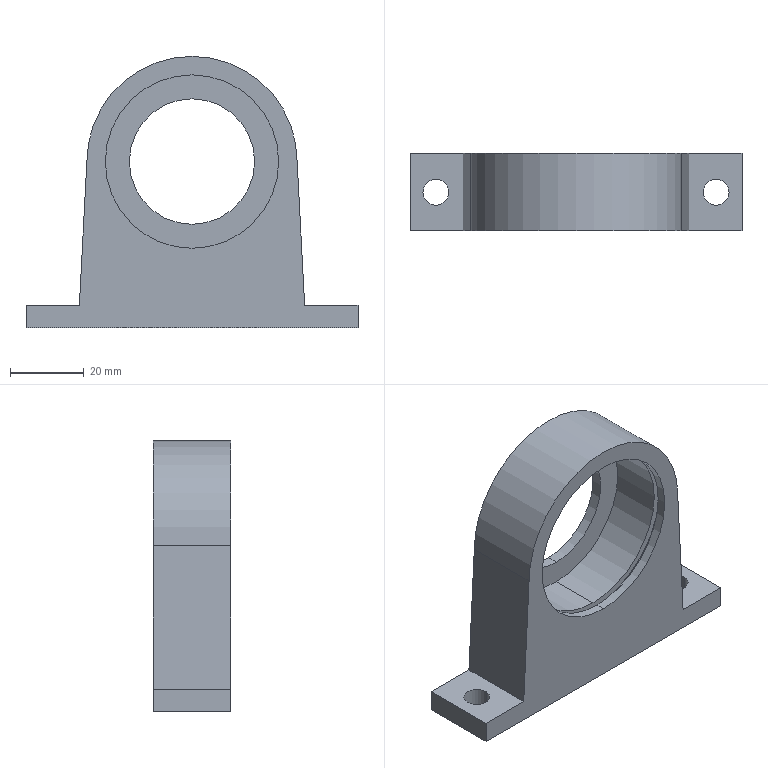Part | STEP file | Floating bearing seat | 1 solid | 25 faces | box 90 x 21 x 73.5 mm | volume 51674 mm3 | cylinder 13 | plane 12 | commonest cylinder face diameters 7 x4 47 x4 34 x2 50.5 x2 57 x1
STEP:
#1=CARTESIAN_POINT('',(0.,-5.5,19.75));
#2=VERTEX_POINT('',#1);
#3=CARTESIAN_POINT('',(0.,-5.5,70.25));
#4=VERTEX_POINT('',#3);
#5=CARTESIAN_POINT('',(0.,-5.5,45.));
#6=DIRECTION('',(0.,1.,0.));
#7=DIRECTION('',(0.,0.,1.));
#8=AXIS2_PLACEMENT_3D('',#5,#6,#7);
#9=CIRCLE('',#8,25.25);
#10=EDGE_CURVE('',#2,#4,#9,.T.);
#11=ORIENTED_EDGE('',*,*,#10,.F.);
#12=CARTESIAN_POINT('',(0.,-4.,19.75));
#13=VERTEX_POINT('',#12);
#14=CARTESIAN_POINT('',(0.,13.,19.75));
#15=DIRECTION('',(0.,1.,0.));
#16=VECTOR('',#15,1000.);
#17=LINE('',#14,#16);
#18=EDGE_CURVE('',#2,#13,#17,.T.);
#19=ORIENTED_EDGE('',*,*,#18,.T.);
#20=CARTESIAN_POINT('',(0.,-4.,70.25));
#21=VERTEX_POINT('',#20);
#22=CARTESIAN_POINT('',(0.,-4.,45.));
#23=DIRECTION('',(0.,1.,0.));
#24=DIRECTION('',(0.,0.,1.));
#25=AXIS2_PLACEMENT_3D('',#22,#23,#24);
#26=CIRCLE('',#25,25.25);
#27=EDGE_CURVE('',#13,#21,#26,.T.);
#28=ORIENTED_EDGE('',*,*,#27,.T.);
#29=CARTESIAN_POINT('',(0.,13.,70.25));
#30=DIRECTION('',(0.,1.,0.));
#31=VECTOR('',#30,1000.);
#32=LINE('',#29,#31);
#33=EDGE_CURVE('',#4,#21,#32,.T.);
#34=ORIENTED_EDGE('',*,*,#33,.F.);
#35=EDGE_LOOP('',(#11,#19,#28,#34));
#36=FACE_OUTER_BOUND('',#35,.T.);
#37=CARTESIAN_POINT('',(0.,13.,45.));
#38=DIRECTION('',(0.,1.,0.));
#39=DIRECTION('',(0.,0.,1.));
#40=AXIS2_PLACEMENT_3D('',#37,#38,#39);
#41=CYLINDRICAL_SURFACE('',#40,25.25);
#42=ADVANCED_FACE('',(#36),#41,.F.);
#43=CARTESIAN_POINT('',(-34.5,2.5,0.));
#44=VERTEX_POINT('',#43);
#45=CARTESIAN_POINT('',(-41.5,2.5,0.));
#46=VERTEX_POINT('',#45);
#47=CARTESIAN_POINT('',(-38.,2.5,0.));
#48=DIRECTION('',(0.,0.,-1.));
#49=DIRECTION('',(1.,0.,0.));
#50=AXIS2_PLACEMENT_3D('',#47,#48,#49);
#51=CIRCLE('',#50,3.5);
#52=EDGE_CURVE('',#44,#46,#51,.T.);
#53=ORIENTED_EDGE('',*,*,#52,.T.);
#54=CARTESIAN_POINT('',(-41.5,2.5,6.));
#55=VERTEX_POINT('',#54);
#56=CARTESIAN_POINT('',(-41.5,2.5,-4.));
#57=DIRECTION('',(0.,0.,1.));
#58=VECTOR('',#57,1000.);
#59=LINE('',#56,#58);
#60=EDGE_CURVE('',#46,#55,#59,.T.);
#61=ORIENTED_EDGE('',*,*,#60,.T.);
#62=CARTESIAN_POINT('',(-34.5,2.5,6.));
#63=VERTEX_POINT('',#62);
#64=CARTESIAN_POINT('',(-38.,2.5,6.));
#65=DIRECTION('',(0.,0.,-1.));
#66=DIRECTION('',(-1.,0.,0.));
#67=AXIS2_PLACEMENT_3D('',#64,#65,#66);
#68=CIRCLE('',#67,3.5);
#69=EDGE_CURVE('',#63,#55,#68,.T.);
#70=ORIENTED_EDGE('',*,*,#69,.F.);
#71=CARTESIAN_POINT('',(-34.5,2.5,-4.));
#72=DIRECTION('',(0.,0.,1.));
#73=VECTOR('',#72,1000.);
#74=LINE('',#71,#73);
#75=EDGE_CURVE('',#44,#63,#74,.T.);
#76=ORIENTED_EDGE('',*,*,#75,.F.);
#77=EDGE_LOOP('',(#53,#61,#70,#76));
#78=FACE_OUTER_BOUND('',#77,.T.);
#79=CARTESIAN_POINT('',(-38.,2.5,-4.));
#80=DIRECTION('',(0.,0.,1.));
#81=DIRECTION('',(1.,0.,0.));
#82=AXIS2_PLACEMENT_3D('',#79,#80,#81);
#83=CYLINDRICAL_SURFACE('',#82,3.5);
#84=ADVANCED_FACE('',(#78),#83,.F.);
#85=CARTESIAN_POINT('',(34.5,2.5,0.));
#86=VERTEX_POINT('',#85);
#87=CARTESIAN_POINT('',(41.5,2.5,0.));
#88=VERTEX_POINT('',#87);
#89=CARTESIAN_POINT('',(38.,2.5,0.));
#90=DIRECTION('',(0.,0.,1.));
#91=DIRECTION('',(1.,0.,0.));
#92=AXIS2_PLACEMENT_3D('',#89,#90,#91);
#93=CIRCLE('',#92,3.5);
#94=EDGE_CURVE('',#86,#88,#93,.T.);
#95=ORIENTED_EDGE('',*,*,#94,.F.);
#96=CARTESIAN_POINT('',(34.5,2.5,6.));
#97=VERTEX_POINT('',#96);
#98=CARTESIAN_POINT('',(34.5,2.5,-4.));
#99=DIRECTION('',(0.,0.,1.));
#100=VECTOR('',#99,1000.);
#101=LINE('',#98,#100);
#102=EDGE_CURVE('',#86,#97,#101,.T.);
#103=ORIENTED_EDGE('',*,*,#102,.T.);
#104=CARTESIAN_POINT('',(41.5,2.5,6.));
#105=VERTEX_POINT('',#104);
#106=CARTESIAN_POINT('',(38.,2.5,6.));
#107=DIRECTION('',(0.,0.,1.));
#108=DIRECTION('',(1.,0.,0.));
#109=AXIS2_PLACEMENT_3D('',#106,#107,#108);
#110=CIRCLE('',#109,3.5);
#111=EDGE_CURVE('',#97,#105,#110,.T.);
#112=ORIENTED_EDGE('',*,*,#111,.T.);
#113=CARTESIAN_POINT('',(41.5,2.5,-4.));
#114=DIRECTION('',(0.,0.,1.));
#115=VECTOR('',#114,1000.);
#116=LINE('',#113,#115);
#117=EDGE_CURVE('',#88,#105,#116,.T.);
#118=ORIENTED_EDGE('',*,*,#117,.F.);
#119=EDGE_LOOP('',(#95,#103,#112,#118));
#120=FACE_OUTER_BOUND('',#119,.T.);
#121=CARTESIAN_POINT('',(38.,2.5,-4.));
#122=DIRECTION('',(0.,0.,1.));
#123=DIRECTION('',(1.,0.,0.));
#124=AXIS2_PLACEMENT_3D('',#121,#122,#123);
#125=CYLINDRICAL_SURFACE('',#124,3.5);
#126=ADVANCED_FACE('',(#120),#125,.F.);
#127=CARTESIAN_POINT('',(0.,10.,68.5));
#128=VERTEX_POINT('',#127);
#129=CARTESIAN_POINT('',(0.,10.,21.5));
#130=VERTEX_POINT('',#129);
#131=CARTESIAN_POINT('',(0.,10.,45.));
#132=DIRECTION('',(0.,-1.,0.));
#133=DIRECTION('',(0.,0.,-1.));
#134=AXIS2_PLACEMENT_3D('',#131,#132,#133);
#135=CIRCLE('',#134,23.5);
#136=EDGE_CURVE('',#128,#130,#135,.T.);
#137=ORIENTED_EDGE('',*,*,#136,.F.);
#138=CARTESIAN_POINT('',(0.,-4.,68.5));
#139=VERTEX_POINT('',#138);
#140=CARTESIAN_POINT('',(0.,8.,68.5));
#141=DIRECTION('',(0.,-1.,0.));
#142=VECTOR('',#141,1000.);
#143=LINE('',#140,#142);
#144=EDGE_CURVE('',#128,#139,#143,.T.);
#145=ORIENTED_EDGE('',*,*,#144,.T.);
#146=CARTESIAN_POINT('',(0.,-4.,21.5));
#147=VERTEX_POINT('',#146);
#148=CARTESIAN_POINT('',(0.,-4.,45.));
#149=DIRECTION('',(0.,1.,0.));
#150=DIRECTION('',(0.,0.,1.));
#151=AXIS2_PLACEMENT_3D('',#148,#149,#150);
#152=CIRCLE('',#151,23.5);
#153=EDGE_CURVE('',#147,#139,#152,.T.);
#154=ORIENTED_EDGE('',*,*,#153,.F.);
#155=CARTESIAN_POINT('',(0.,8.,21.5));
#156=DIRECTION('',(0.,-1.,0.));
#157=VECTOR('',#156,1000.);
#158=LINE('',#155,#157);
#159=EDGE_CURVE('',#130,#147,#158,.T.);
#160=ORIENTED_EDGE('',*,*,#159,.F.);
#161=EDGE_LOOP('',(#137,#145,#154,#160));
#162=FACE_OUTER_BOUND('',#161,.T.);
#163=CARTESIAN_POINT('',(0.,8.,45.));
#164=DIRECTION('',(0.,-1.,0.));
#165=DIRECTION('',(0.,0.,-1.));
#166=AXIS2_PLACEMENT_3D('',#163,#164,#165);
#167=CYLINDRICAL_SURFACE('',#166,23.5);
#168=ADVANCED_FACE('',(#162),#167,.F.);
#169=CARTESIAN_POINT('',(0.,13.,28.));
#170=VERTEX_POINT('',#169);
#171=CARTESIAN_POINT('',(0.,13.,62.));
#172=VERTEX_POINT('',#171);
#173=CARTESIAN_POINT('',(0.,13.,45.));
#174=DIRECTION('',(0.,1.,0.));
#175=DIRECTION('',(0.,0.,1.));
#176=AXIS2_PLACEMENT_3D('',#173,#174,#175);
#177=CIRCLE('',#176,17.);
#178=EDGE_CURVE('',#170,#172,#177,.T.);
#179=ORIENTED_EDGE('',*,*,#178,.T.);
#180=CARTESIAN_POINT('',(0.,10.,62.));
#181=VERTEX_POINT('',#180);
#182=CARTESIAN_POINT('',(0.,13.,62.));
#183=DIRECTION('',(0.,-1.,0.));
#184=VECTOR('',#183,1000.);
#185=LINE('',#182,#184);
#186=EDGE_CURVE('',#172,#181,#185,.T.);
#187=ORIENTED_EDGE('',*,*,#186,.T.);
#188=CARTESIAN_POINT('',(0.,10.,28.));
#189=VERTEX_POINT('',#188);
#190=CARTESIAN_POINT('',(0.,10.,45.));
#191=DIRECTION('',(0.,-1.,0.));
#192=DIRECTION('',(0.,0.,-1.));
#193=AXIS2_PLACEMENT_3D('',#190,#191,#192);
#194=CIRCLE('',#193,17.);
#195=EDGE_CURVE('',#181,#189,#194,.T.);
#196=ORIENTED_EDGE('',*,*,#195,.T.);
#197=CARTESIAN_POINT('',(0.,13.,28.));
#198=DIRECTION('',(0.,-1.,0.));
#199=VECTOR('',#198,1000.);
#200=LINE('',#197,#199);
#201=EDGE_CURVE('',#170,#189,#200,.T.);
#202=ORIENTED_EDGE('',*,*,#201,.F.);
#203=EDGE_LOOP('',(#179,#187,#196,#202));
#204=FACE_OUTER_BOUND('',#203,.T.);
#205=CARTESIAN_POINT('',(0.,13.,45.));
#206=DIRECTION('',(0.,-1.,0.));
#207=DIRECTION('',(0.,0.,-1.));
#208=AXIS2_PLACEMENT_3D('',#205,#206,#207);
#209=CYLINDRICAL_SURFACE('',#208,17.);
#210=ADVANCED_FACE('',(#204),#209,.F.);
#211=CARTESIAN_POINT('',(0.,-5.5,68.5));
#212=VERTEX_POINT('',#211);
#213=CARTESIAN_POINT('',(0.,-5.5,21.5));
#214=VERTEX_POINT('',#213);
#215=CARTESIAN_POINT('',(0.,-5.5,45.));
#216=DIRECTION('',(0.,-1.,0.));
#217=DIRECTION('',(0.,0.,-1.));
#218=AXIS2_PLACEMENT_3D('',#215,#216,#217);
#219=CIRCLE('',#218,23.5);
#220=EDGE_CURVE('',#212,#214,#219,.T.);
#221=ORIENTED_EDGE('',*,*,#220,.F.);
#222=CARTESIAN_POINT('',(0.,-8.,68.5));
#223=VERTEX_POINT('',#222);
#224=CARTESIAN_POINT('',(0.,8.,68.5));
#225=DIRECTION('',(0.,-1.,0.));
#226=VECTOR('',#225,1000.);
#227=LINE('',#224,#226);
#228=EDGE_CURVE('',#212,#223,#227,.T.);
#229=ORIENTED_EDGE('',*,*,#228,.T.);
#230=CARTESIAN_POINT('',(0.,-8.,21.5));
#231=VERTEX_POINT('',#230);
#232=CARTESIAN_POINT('',(0.,-8.,45.));
#233=DIRECTION('',(0.,1.,0.));
#234=DIRECTION('',(0.,0.,1.));
#235=AXIS2_PLACEMENT_3D('',#232,#233,#234);
#236=CIRCLE('',#235,23.5);
#237=EDGE_CURVE('',#231,#223,#236,.T.);
#238=ORIENTED_EDGE('',*,*,#237,.F.);
#239=CARTESIAN_POINT('',(0.,8.,21.5));
#240=DIRECTION('',(0.,-1.,0.));
#241=VECTOR('',#240,1000.);
#242=LINE('',#239,#241);
#243=EDGE_CURVE('',#214,#231,#242,.T.);
#244=ORIENTED_EDGE('',*,*,#243,.F.);
#245=EDGE_LOOP('',(#221,#229,#238,#244));
#246=FACE_OUTER_BOUND('',#245,.T.);
#247=CARTESIAN_POINT('',(0.,8.,45.));
#248=DIRECTION('',(0.,-1.,0.));
#249=DIRECTION('',(0.,0.,-1.));
#250=AXIS2_PLACEMENT_3D('',#247,#248,#249);
#251=CYLINDRICAL_SURFACE('',#250,23.5);
#252=ADVANCED_FACE('',(#246),#251,.F.);
#253=ORIENTED_EDGE('',*,*,#228,.F.);
#254=CARTESIAN_POINT('',(0.,-5.5,45.));
#255=DIRECTION('',(0.,-1.,0.));
#256=DIRECTION('',(0.,0.,-1.));
#257=AXIS2_PLACEMENT_3D('',#254,#255,#256);
#258=CIRCLE('',#257,23.5);
#259=EDGE_CURVE('',#214,#212,#258,.T.);
#260=ORIENTED_EDGE('',*,*,#259,.F.);
#261=ORIENTED_EDGE('',*,*,#243,.T.);
#262=CARTESIAN_POINT('',(0.,-8.,45.));
#263=DIRECTION('',(0.,1.,0.));
#264=DIRECTION('',(0.,0.,1.));
#265=AXIS2_PLACEMENT_3D('',#262,#263,#264);
#266=CIRCLE('',#265,23.5);
#267=EDGE_CURVE('',#223,#231,#266,.T.);
#268=ORIENTED_EDGE('',*,*,#267,.F.);
#269=EDGE_LOOP('',(#253,#260,#261,#268));
#270=FACE_OUTER_BOUND('',#269,.T.);
#271=CARTESIAN_POINT('',(0.,8.,45.));
#272=DIRECTION('',(0.,-1.,0.));
#273=DIRECTION('',(0.,0.,-1.));
#274=AXIS2_PLACEMENT_3D('',#271,#272,#273);
#275=CYLINDRICAL_SURFACE('',#274,23.5);
#276=ADVANCED_FACE('',(#270),#275,.F.);
#277=ORIENTED_EDGE('',*,*,#186,.F.);
#278=CARTESIAN_POINT('',(0.,13.,45.));
#279=DIRECTION('',(0.,1.,0.));
#280=DIRECTION('',(0.,0.,1.));
#281=AXIS2_PLACEMENT_3D('',#278,#279,#280);
#282=CIRCLE('',#281,17.);
#283=EDGE_CURVE('',#172,#170,#282,.T.);
#284=ORIENTED_EDGE('',*,*,#283,.T.);
#285=ORIENTED_EDGE('',*,*,#201,.T.);
#286=CARTESIAN_POINT('',(0.,10.,45.));
#287=DIRECTION('',(0.,-1.,0.));
#288=DIRECTION('',(0.,0.,-1.));
#289=AXIS2_PLACEMENT_3D('',#286,#287,#288);
#290=CIRCLE('',#289,17.);
#291=EDGE_CURVE('',#189,#181,#290,.T.);
#292=ORIENTED_EDGE('',*,*,#291,.T.);
#293=EDGE_LOOP('',(#277,#284,#285,#292));
#294=FACE_OUTER_BOUND('',#293,.T.);
#295=CARTESIAN_POINT('',(0.,13.,45.));
#296=DIRECTION('',(0.,-1.,0.));
#297=DIRECTION('',(0.,0.,-1.));
#298=AXIS2_PLACEMENT_3D('',#295,#296,#297);
#299=CYLINDRICAL_SURFACE('',#298,17.);
#300=ADVANCED_FACE('',(#294),#299,.F.);
#301=ORIENTED_EDGE('',*,*,#69,.T.);
#302=CARTESIAN_POINT('',(-38.,2.5,6.));
#303=DIRECTION('',(0.,0.,-1.));
#304=DIRECTION('',(-1.,0.,0.));
#305=AXIS2_PLACEMENT_3D('',#302,#303,#304);
#306=CIRCLE('',#305,3.5);
#307=EDGE_CURVE('',#55,#63,#306,.T.);
#308=ORIENTED_EDGE('',*,*,#307,.T.);
#309=EDGE_LOOP('',(#301,#308));
#310=FACE_BOUND('',#309,.T.);
#311=CARTESIAN_POINT('',(-45.,-8.,6.));
#312=VERTEX_POINT('',#311);
#313=CARTESIAN_POINT('',(-45.,13.,6.));
#314=VERTEX_POINT('',#313);
#315=CARTESIAN_POINT('',(-45.,-24.,6.));
#316=DIRECTION('',(0.,1.,0.));
#317=VECTOR('',#316,1000.);
#318=LINE('',#315,#317);
#319=EDGE_CURVE('',#312,#314,#318,.T.);
#320=ORIENTED_EDGE('',*,*,#319,.F.);
#321=CARTESIAN_POINT('',(-30.544,-8.,6.));
#322=VERTEX_POINT('',#321);
#323=CARTESIAN_POINT('',(45.,-8.,6.));
#324=DIRECTION('',(-1.,0.,0.));
#325=VECTOR('',#324,1000.);
#326=LINE('',#323,#325);
#327=EDGE_CURVE('',#322,#312,#326,.T.);
#328=ORIENTED_EDGE('',*,*,#327,.F.);
#329=CARTESIAN_POINT('',(-30.544,13.,6.));
#330=VERTEX_POINT('',#329);
#331=CARTESIAN_POINT('',(-30.544,0.,6.));
#332=DIRECTION('',(0.,1.,0.));
#333=VECTOR('',#332,1000.);
#334=LINE('',#331,#333);
#335=EDGE_CURVE('',#322,#330,#334,.T.);
#336=ORIENTED_EDGE('',*,*,#335,.T.);
#337=CARTESIAN_POINT('',(-34.,13.,6.));
#338=DIRECTION('',(1.,0.,0.));
#339=VECTOR('',#338,1000.);
#340=LINE('',#337,#339);
#341=EDGE_CURVE('',#314,#330,#340,.T.);
#342=ORIENTED_EDGE('',*,*,#341,.F.);
#343=EDGE_LOOP('',(#320,#328,#336,#342));
#344=FACE_OUTER_BOUND('',#343,.T.);
#345=CARTESIAN_POINT('',(0.,0.,6.));
#346=DIRECTION('',(0.,0.,1.));
#347=DIRECTION('',(1.,0.,0.));
#348=AXIS2_PLACEMENT_3D('',#345,#346,#347);
#349=PLANE('',#348);
#350=ADVANCED_FACE('',(#310,#344),#349,.T.);
#351=CARTESIAN_POINT('',(38.,2.5,6.));
#352=DIRECTION('',(0.,0.,1.));
#353=DIRECTION('',(1.,0.,0.));
#354=AXIS2_PLACEMENT_3D('',#351,#352,#353);
#355=CIRCLE('',#354,3.5);
#356=EDGE_CURVE('',#105,#97,#355,.T.);
#357=ORIENTED_EDGE('',*,*,#356,.F.);
#358=ORIENTED_EDGE('',*,*,#111,.F.);
#359=EDGE_LOOP('',(#357,#358));
#360=FACE_BOUND('',#359,.T.);
#361=CARTESIAN_POINT('',(30.544,13.,6.));
#362=VERTEX_POINT('',#361);
#363=CARTESIAN_POINT('',(30.544,-8.,6.));
#364=VERTEX_POINT('',#363);
#365=CARTESIAN_POINT('',(30.544,0.,6.));
#366=DIRECTION('',(0.,-1.,0.));
#367=VECTOR('',#366,1000.);
#368=LINE('',#365,#367);
#369=EDGE_CURVE('',#362,#364,#368,.T.);
#370=ORIENTED_EDGE('',*,*,#369,.T.);
#371=CARTESIAN_POINT('',(45.,-8.,6.));
#372=VERTEX_POINT('',#371);
#373=CARTESIAN_POINT('',(45.,-8.,6.));
#374=DIRECTION('',(-1.,0.,0.));
#375=VECTOR('',#374,1000.);
#376=LINE('',#373,#375);
#377=EDGE_CURVE('',#372,#364,#376,.T.);
#378=ORIENTED_EDGE('',*,*,#377,.F.);
#379=CARTESIAN_POINT('',(45.,13.,6.));
#380=VERTEX_POINT('',#379);
#381=CARTESIAN_POINT('',(45.,13.,6.));
#382=DIRECTION('',(0.,-1.,0.));
#383=VECTOR('',#382,1000.);
#384=LINE('',#381,#383);
#385=EDGE_CURVE('',#380,#372,#384,.T.);
#386=ORIENTED_EDGE('',*,*,#385,.F.);
#387=CARTESIAN_POINT('',(-34.,13.,6.));
#388=DIRECTION('',(1.,0.,0.));
#389=VECTOR('',#388,1000.);
#390=LINE('',#387,#389);
#391=EDGE_CURVE('',#362,#380,#390,.T.);
#392=ORIENTED_EDGE('',*,*,#391,.F.);
#393=EDGE_LOOP('',(#370,#378,#386,#392));
#394=FACE_OUTER_BOUND('',#393,.T.);
#395=CARTESIAN_POINT('',(0.,0.,6.));
#396=DIRECTION('',(0.,0.,1.));
#397=DIRECTION('',(1.,0.,0.));
#398=AXIS2_PLACEMENT_3D('',#395,#396,#397);
#399=PLANE('',#398);
#400=ADVANCED_FACE('',(#360,#394),#399,.T.);
#401=ORIENTED_EDGE('',*,*,#52,.F.);
#402=CARTESIAN_POINT('',(-38.,2.5,0.));
#403=DIRECTION('',(0.,0.,-1.));
#404=DIRECTION('',(1.,0.,0.));
#405=AXIS2_PLACEMENT_3D('',#402,#403,#404);
#406=CIRCLE('',#405,3.5);
#407=EDGE_CURVE('',#46,#44,#406,.T.);
#408=ORIENTED_EDGE('',*,*,#407,.F.);
#409=EDGE_LOOP('',(#401,#408));
#410=FACE_BOUND('',#409,.T.);
#411=CARTESIAN_POINT('',(38.,2.5,0.));
#412=DIRECTION('',(0.,0.,1.));
#413=DIRECTION('',(1.,0.,0.));
#414=AXIS2_PLACEMENT_3D('',#411,#412,#413);
#415=CIRCLE('',#414,3.5);
#416=EDGE_CURVE('',#88,#86,#415,.T.);
#417=ORIENTED_EDGE('',*,*,#416,.T.);
#418=ORIENTED_EDGE('',*,*,#94,.T.);
#419=EDGE_LOOP('',(#417,#418));
#420=FACE_BOUND('',#419,.T.);
#421=CARTESIAN_POINT('',(-45.,-8.,0.));
#422=VERTEX_POINT('',#421);
#423=CARTESIAN_POINT('',(45.,-8.,0.));
#424=VERTEX_POINT('',#423);
#425=CARTESIAN_POINT('',(-45.,-8.,0.));
#426=DIRECTION('',(1.,0.,0.));
#427=VECTOR('',#426,1000.);
#428=LINE('',#425,#427);
#429=EDGE_CURVE('',#422,#424,#428,.T.);
#430=ORIENTED_EDGE('',*,*,#429,.F.);
#431=CARTESIAN_POINT('',(-45.,13.,0.));
#432=VERTEX_POINT('',#431);
#433=CARTESIAN_POINT('',(-45.,13.,0.));
#434=DIRECTION('',(0.,-1.,0.));
#435=VECTOR('',#434,1000.);
#436=LINE('',#433,#435);
#437=EDGE_CURVE('',#432,#422,#436,.T.);
#438=ORIENTED_EDGE('',*,*,#437,.F.);
#439=CARTESIAN_POINT('',(45.,13.,0.));
#440=VERTEX_POINT('',#439);
#441=CARTESIAN_POINT('',(34.,13.,0.));
#442=DIRECTION('',(-1.,0.,0.));
#443=VECTOR('',#442,1000.);
#444=LINE('',#441,#443);
#445=EDGE_CURVE('',#440,#432,#444,.T.);
#446=ORIENTED_EDGE('',*,*,#445,.F.);
#447=CARTESIAN_POINT('',(45.,-24.,0.));
#448=DIRECTION('',(0.,1.,0.));
#449=VECTOR('',#448,1000.);
#450=LINE('',#447,#449);
#451=EDGE_CURVE('',#424,#440,#450,.T.);
#452=ORIENTED_EDGE('',*,*,#451,.F.);
#453=EDGE_LOOP('',(#430,#438,#446,#452));
#454=FACE_OUTER_BOUND('',#453,.T.);
#455=CARTESIAN_POINT('',(0.,0.,0.));
#456=DIRECTION('',(0.,0.,1.));
#457=DIRECTION('',(1.,0.,0.));
#458=AXIS2_PLACEMENT_3D('',#455,#456,#457);
#459=PLANE('',#458);
#460=ADVANCED_FACE('',(#410,#420,#454),#459,.F.);
#461=ORIENTED_EDGE('',*,*,#437,.T.);
#462=CARTESIAN_POINT('',(-45.,-8.,6.));
#463=DIRECTION('',(0.,0.,-1.));
#464=VECTOR('',#463,1000.);
#465=LINE('',#462,#464);
#466=EDGE_CURVE('',#312,#422,#465,.T.);
#467=ORIENTED_EDGE('',*,*,#466,.F.);
#468=ORIENTED_EDGE('',*,*,#319,.T.);
#469=CARTESIAN_POINT('',(-45.,13.,6.));
#470=DIRECTION('',(0.,0.,-1.));
#471=VECTOR('',#470,1000.);
#472=LINE('',#469,#471);
#473=EDGE_CURVE('',#314,#432,#472,.T.);
#474=ORIENTED_EDGE('',*,*,#473,.T.);
#475=EDGE_LOOP('',(#461,#467,#468,#474));
#476=FACE_OUTER_BOUND('',#475,.T.);
#477=CARTESIAN_POINT('',(-45.,0.,0.));
#478=DIRECTION('',(-1.,0.,0.));
#479=DIRECTION('',(0.,0.,1.));
#480=AXIS2_PLACEMENT_3D('',#477,#478,#479);
#481=PLANE('',#480);
#482=ADVANCED_FACE('',(#476),#481,.T.);
#483=ORIENTED_EDGE('',*,*,#385,.T.);
#484=CARTESIAN_POINT('',(45.,-8.,0.));
#485=DIRECTION('',(0.,0.,1.));
#486=VECTOR('',#485,1000.);
#487=LINE('',#484,#486);
#488=EDGE_CURVE('',#424,#372,#487,.T.);
#489=ORIENTED_EDGE('',*,*,#488,.F.);
#490=ORIENTED_EDGE('',*,*,#451,.T.);
#491=CARTESIAN_POINT('',(45.,13.,0.));
#492=DIRECTION('',(0.,0.,1.));
#493=VECTOR('',#492,1000.);
#494=LINE('',#491,#493);
#495=EDGE_CURVE('',#440,#380,#494,.T.);
#496=ORIENTED_EDGE('',*,*,#495,.T.);
#497=EDGE_LOOP('',(#483,#489,#490,#496));
#498=FACE_OUTER_BOUND('',#497,.T.);
#499=CARTESIAN_POINT('',(45.,0.,0.));
#500=DIRECTION('',(1.,0.,0.));
#501=DIRECTION('',(0.,0.,-1.));
#502=AXIS2_PLACEMENT_3D('',#499,#500,#501);
#503=PLANE('',#502);
#504=ADVANCED_FACE('',(#498),#503,.T.);
#505=CARTESIAN_POINT('',(-28.5,-8.,45.));
#506=VERTEX_POINT('',#505);
#507=CARTESIAN_POINT('',(-28.5,-8.,45.));
#508=DIRECTION('',(0.05234,0.,0.9986));
#509=VECTOR('',#508,1000.);
#510=LINE('',#507,#509);
#511=EDGE_CURVE('',#322,#506,#510,.T.);
#512=ORIENTED_EDGE('',*,*,#511,.F.);
#513=ORIENTED_EDGE('',*,*,#327,.T.);
#514=ORIENTED_EDGE('',*,*,#466,.T.);
#515=ORIENTED_EDGE('',*,*,#429,.T.);
#516=ORIENTED_EDGE('',*,*,#488,.T.);
#517=ORIENTED_EDGE('',*,*,#377,.T.);
#518=CARTESIAN_POINT('',(28.5,-8.,45.));
#519=VERTEX_POINT('',#518);
#520=CARTESIAN_POINT('',(28.5,-8.,45.));
#521=DIRECTION('',(0.05234,0.,-0.9986));
#522=VECTOR('',#521,1000.);
#523=LINE('',#520,#522);
#524=EDGE_CURVE('',#519,#364,#523,.T.);
#525=ORIENTED_EDGE('',*,*,#524,.F.);
#526=CARTESIAN_POINT('',(0.,-8.,45.));
#527=DIRECTION('',(0.,1.,0.));
#528=DIRECTION('',(0.,0.,1.));
#529=AXIS2_PLACEMENT_3D('',#526,#527,#528);
#530=CIRCLE('',#529,28.5);
#531=EDGE_CURVE('',#506,#519,#530,.T.);
#532=ORIENTED_EDGE('',*,*,#531,.F.);
#533=EDGE_LOOP('',(#512,#513,#514,#515,#516,#517,#525,#532));
#534=FACE_OUTER_BOUND('',#533,.T.);
#535=ORIENTED_EDGE('',*,*,#237,.T.);
#536=ORIENTED_EDGE('',*,*,#267,.T.);
#537=EDGE_LOOP('',(#535,#536));
#538=FACE_BOUND('',#537,.T.);
#539=CARTESIAN_POINT('',(0.,-8.,45.));
#540=DIRECTION('',(0.,1.,0.));
#541=DIRECTION('',(0.,0.,1.));
#542=AXIS2_PLACEMENT_3D('',#539,#540,#541);
#543=PLANE('',#542);
#544=ADVANCED_FACE('',(#534,#538),#543,.F.);
#545=ORIENTED_EDGE('',*,*,#531,.T.);
#546=CARTESIAN_POINT('',(28.5,13.,45.));
#547=VERTEX_POINT('',#546);
#548=CARTESIAN_POINT('',(28.5,8.,45.));
#549=DIRECTION('',(0.,-1.,0.));
#550=VECTOR('',#549,1000.);
#551=LINE('',#548,#550);
#552=EDGE_CURVE('',#547,#519,#551,.T.);
#553=ORIENTED_EDGE('',*,*,#552,.F.);
#554=CARTESIAN_POINT('',(-28.5,13.,45.));
#555=VERTEX_POINT('',#554);
#556=CARTESIAN_POINT('',(0.,13.,45.));
#557=DIRECTION('',(0.,1.,0.));
#558=DIRECTION('',(0.,0.,1.));
#559=AXIS2_PLACEMENT_3D('',#556,#557,#558);
#560=CIRCLE('',#559,28.5);
#561=EDGE_CURVE('',#555,#547,#560,.T.);
#562=ORIENTED_EDGE('',*,*,#561,.F.);
#563=CARTESIAN_POINT('',(-28.5,8.,45.));
#564=DIRECTION('',(0.,-1.,0.));
#565=VECTOR('',#564,1000.);
#566=LINE('',#563,#565);
#567=EDGE_CURVE('',#555,#506,#566,.T.);
#568=ORIENTED_EDGE('',*,*,#567,.T.);
#569=EDGE_LOOP('',(#545,#553,#562,#568));
#570=FACE_OUTER_BOUND('',#569,.T.);
#571=CARTESIAN_POINT('',(0.,8.,45.));
#572=DIRECTION('',(0.,-1.,0.));
#573=DIRECTION('',(0.,0.,-1.));
#574=AXIS2_PLACEMENT_3D('',#571,#572,#573);
#575=CYLINDRICAL_SURFACE('',#574,28.5);
#576=ADVANCED_FACE('',(#570),#575,.T.);
#577=ORIENTED_EDGE('',*,*,#369,.F.);
#578=CARTESIAN_POINT('',(28.5,13.,45.));
#579=DIRECTION('',(0.05234,0.,-0.9986));
#580=VECTOR('',#579,1000.);
#581=LINE('',#578,#580);
#582=EDGE_CURVE('',#547,#362,#581,.T.);
#583=ORIENTED_EDGE('',*,*,#582,.F.);
#584=ORIENTED_EDGE('',*,*,#552,.T.);
#585=ORIENTED_EDGE('',*,*,#524,.T.);
#586=EDGE_LOOP('',(#577,#583,#584,#585));
#587=FACE_OUTER_BOUND('',#586,.T.);
#588=CARTESIAN_POINT('',(28.5,8.,45.));
#589=DIRECTION('',(-0.9986,0.,-0.05234));
#590=DIRECTION('',(-0.05234,0.,0.9986));
#591=AXIS2_PLACEMENT_3D('',#588,#589,#590);
#592=PLANE('',#591);
#593=ADVANCED_FACE('',(#587),#592,.F.);
#594=ORIENTED_EDGE('',*,*,#335,.F.);
#595=ORIENTED_EDGE('',*,*,#511,.T.);
#596=ORIENTED_EDGE('',*,*,#567,.F.);
#597=CARTESIAN_POINT('',(-30.544,13.,6.));
#598=DIRECTION('',(0.05234,0.,0.9986));
#599=VECTOR('',#598,1000.);
#600=LINE('',#597,#599);
#601=EDGE_CURVE('',#330,#555,#600,.T.);
#602=ORIENTED_EDGE('',*,*,#601,.F.);
#603=EDGE_LOOP('',(#594,#595,#596,#602));
#604=FACE_OUTER_BOUND('',#603,.T.);
#605=CARTESIAN_POINT('',(-28.5,8.,45.));
#606=DIRECTION('',(0.9986,0.,-0.05234));
#607=DIRECTION('',(-0.05234,0.,-0.9986));
#608=AXIS2_PLACEMENT_3D('',#605,#606,#607);
#609=PLANE('',#608);
#610=ADVANCED_FACE('',(#604),#609,.F.);
#611=ORIENTED_EDGE('',*,*,#144,.F.);
#612=CARTESIAN_POINT('',(0.,10.,45.));
#613=DIRECTION('',(0.,-1.,0.));
#614=DIRECTION('',(0.,0.,-1.));
#615=AXIS2_PLACEMENT_3D('',#612,#613,#614);
#616=CIRCLE('',#615,23.5);
#617=EDGE_CURVE('',#130,#128,#616,.T.);
#618=ORIENTED_EDGE('',*,*,#617,.F.);
#619=ORIENTED_EDGE('',*,*,#159,.T.);
#620=CARTESIAN_POINT('',(0.,-4.,45.));
#621=DIRECTION('',(0.,1.,0.));
#622=DIRECTION('',(0.,0.,1.));
#623=AXIS2_PLACEMENT_3D('',#620,#621,#622);
#624=CIRCLE('',#623,23.5);
#625=EDGE_CURVE('',#139,#147,#624,.T.);
#626=ORIENTED_EDGE('',*,*,#625,.F.);
#627=EDGE_LOOP('',(#611,#618,#619,#626));
#628=FACE_OUTER_BOUND('',#627,.T.);
#629=CARTESIAN_POINT('',(0.,8.,45.));
#630=DIRECTION('',(0.,-1.,0.));
#631=DIRECTION('',(0.,0.,-1.));
#632=AXIS2_PLACEMENT_3D('',#629,#630,#631);
#633=CYLINDRICAL_SURFACE('',#632,23.5);
#634=ADVANCED_FACE('',(#628),#633,.F.);
#635=ORIENTED_EDGE('',*,*,#561,.T.);
#636=ORIENTED_EDGE('',*,*,#582,.T.);
#637=ORIENTED_EDGE('',*,*,#391,.T.);
#638=ORIENTED_EDGE('',*,*,#495,.F.);
#639=ORIENTED_EDGE('',*,*,#445,.T.);
#640=ORIENTED_EDGE('',*,*,#473,.F.);
#641=ORIENTED_EDGE('',*,*,#341,.T.);
#642=ORIENTED_EDGE('',*,*,#601,.T.);
#643=EDGE_LOOP('',(#635,#636,#637,#638,#639,#640,#641,#642));
#644=FACE_OUTER_BOUND('',#643,.T.);
#645=ORIENTED_EDGE('',*,*,#178,.F.);
#646=ORIENTED_EDGE('',*,*,#283,.F.);
#647=EDGE_LOOP('',(#645,#646));
#648=FACE_BOUND('',#647,.T.);
#649=CARTESIAN_POINT('',(0.,13.,45.));
#650=DIRECTION('',(0.,1.,0.));
#651=DIRECTION('',(0.,0.,1.));
#652=AXIS2_PLACEMENT_3D('',#649,#650,#651);
#653=PLANE('',#652);
#654=ADVANCED_FACE('',(#644,#648),#653,.T.);
#655=ORIENTED_EDGE('',*,*,#102,.F.);
#656=ORIENTED_EDGE('',*,*,#416,.F.);
#657=ORIENTED_EDGE('',*,*,#117,.T.);
#658=ORIENTED_EDGE('',*,*,#356,.T.);
#659=EDGE_LOOP('',(#655,#656,#657,#658));
#660=FACE_OUTER_BOUND('',#659,.T.);
#661=CARTESIAN_POINT('',(38.,2.5,-4.));
#662=DIRECTION('',(0.,0.,1.));
#663=DIRECTION('',(1.,0.,0.));
#664=AXIS2_PLACEMENT_3D('',#661,#662,#663);
#665=CYLINDRICAL_SURFACE('',#664,3.5);
#666=ADVANCED_FACE('',(#660),#665,.F.);
#667=ORIENTED_EDGE('',*,*,#60,.F.);
#668=ORIENTED_EDGE('',*,*,#407,.T.);
#669=ORIENTED_EDGE('',*,*,#75,.T.);
#670=ORIENTED_EDGE('',*,*,#307,.F.);
#671=EDGE_LOOP('',(#667,#668,#669,#670));
#672=FACE_OUTER_BOUND('',#671,.T.);
#673=CARTESIAN_POINT('',(-38.,2.5,-4.));
#674=DIRECTION('',(0.,0.,1.));
#675=DIRECTION('',(1.,0.,0.));
#676=AXIS2_PLACEMENT_3D('',#673,#674,#675);
#677=CYLINDRICAL_SURFACE('',#676,3.5);
#678=ADVANCED_FACE('',(#672),#677,.F.);
#679=ORIENTED_EDGE('',*,*,#291,.F.);
#680=ORIENTED_EDGE('',*,*,#195,.F.);
#681=EDGE_LOOP('',(#679,#680));
#682=FACE_BOUND('',#681,.T.);
#683=ORIENTED_EDGE('',*,*,#617,.T.);
#684=ORIENTED_EDGE('',*,*,#136,.T.);
#685=EDGE_LOOP('',(#683,#684));
#686=FACE_OUTER_BOUND('',#685,.T.);
#687=CARTESIAN_POINT('',(0.,10.,45.));
#688=DIRECTION('',(0.,-1.,0.));
#689=DIRECTION('',(0.,0.,-1.));
#690=AXIS2_PLACEMENT_3D('',#687,#688,#689);
#691=PLANE('',#690);
#692=ADVANCED_FACE('',(#682,#686),#691,.T.);
#693=ORIENTED_EDGE('',*,*,#18,.F.);
#694=CARTESIAN_POINT('',(0.,-5.5,45.));
#695=DIRECTION('',(0.,1.,0.));
#696=DIRECTION('',(0.,0.,1.));
#697=AXIS2_PLACEMENT_3D('',#694,#695,#696);
#698=CIRCLE('',#697,25.25);
#699=EDGE_CURVE('',#4,#2,#698,.T.);
#700=ORIENTED_EDGE('',*,*,#699,.F.);
#701=ORIENTED_EDGE('',*,*,#33,.T.);
#702=CARTESIAN_POINT('',(0.,-4.,45.));
#703=DIRECTION('',(0.,1.,0.));
#704=DIRECTION('',(0.,0.,1.));
#705=AXIS2_PLACEMENT_3D('',#702,#703,#704);
#706=CIRCLE('',#705,25.25);
#707=EDGE_CURVE('',#21,#13,#706,.T.);
#708=ORIENTED_EDGE('',*,*,#707,.T.);
#709=EDGE_LOOP('',(#693,#700,#701,#708));
#710=FACE_OUTER_BOUND('',#709,.T.);
#711=CARTESIAN_POINT('',(0.,13.,45.));
#712=DIRECTION('',(0.,1.,0.));
#713=DIRECTION('',(0.,0.,1.));
#714=AXIS2_PLACEMENT_3D('',#711,#712,#713);
#715=CYLINDRICAL_SURFACE('',#714,25.25);
#716=ADVANCED_FACE('',(#710),#715,.F.);
#717=ORIENTED_EDGE('',*,*,#259,.T.);
#718=ORIENTED_EDGE('',*,*,#220,.T.);
#719=EDGE_LOOP('',(#717,#718));
#720=FACE_BOUND('',#719,.T.);
#721=ORIENTED_EDGE('',*,*,#699,.T.);
#722=ORIENTED_EDGE('',*,*,#10,.T.);
#723=EDGE_LOOP('',(#721,#722));
#724=FACE_OUTER_BOUND('',#723,.T.);
#725=CARTESIAN_POINT('',(0.,-5.5,70.25));
#726=DIRECTION('',(0.,-1.,0.));
#727=DIRECTION('',(0.,0.,-1.));
#728=AXIS2_PLACEMENT_3D('',#725,#726,#727);
#729=PLANE('',#728);
#730=ADVANCED_FACE('',(#720,#724),#729,.F.);
#731=ORIENTED_EDGE('',*,*,#153,.T.);
#732=ORIENTED_EDGE('',*,*,#625,.T.);
#733=EDGE_LOOP('',(#731,#732));
#734=FACE_BOUND('',#733,.T.);
#735=ORIENTED_EDGE('',*,*,#707,.F.);
#736=ORIENTED_EDGE('',*,*,#27,.F.);
#737=EDGE_LOOP('',(#735,#736));
#738=FACE_OUTER_BOUND('',#737,.T.);
#739=CARTESIAN_POINT('',(0.,-4.,70.25));
#740=DIRECTION('',(0.,1.,0.));
#741=DIRECTION('',(0.,0.,1.));
#742=AXIS2_PLACEMENT_3D('',#739,#740,#741);
#743=PLANE('',#742);
#744=ADVANCED_FACE('',(#734,#738),#743,.F.);
#745=CLOSED_SHELL('',(#42,#84,#126,#168,#210,#252,#276,#300,#350,#400,#460,#482,#504,#544,#576,#593,#610,#634,#654,#666,#678,#692,#716,#730,#744));
#746=MANIFOLD_SOLID_BREP('',#745);
#747=CARTESIAN_POINT('',(0.,0.,0.));
#748=DIRECTION('',(0.,0.,1.));
#749=DIRECTION('',(1.,0.,0.));
#750=AXIS2_PLACEMENT_3D('',#747,#748,#749);
#751=(LENGTH_UNIT()NAMED_UNIT(*)SI_UNIT(.MILLI.,.METRE.));
#752=UNCERTAINTY_MEASURE_WITH_UNIT(LENGTH_MEASURE(0.00001),#751,'','');
#753=(NAMED_UNIT(*)PLANE_ANGLE_UNIT()SI_UNIT($,.RADIAN.));
#754=(NAMED_UNIT(*)SI_UNIT($,.STERADIAN.)SOLID_ANGLE_UNIT());
#755=(GEOMETRIC_REPRESENTATION_CONTEXT(3)GLOBAL_UNCERTAINTY_ASSIGNED_CONTEXT((#752))GLOBAL_UNIT_ASSIGNED_CONTEXT((#751,#753,#754))REPRESENTATION_CONTEXT('',''));
#756=ADVANCED_BREP_SHAPE_REPRESENTATION('',(#746,#750),#755);